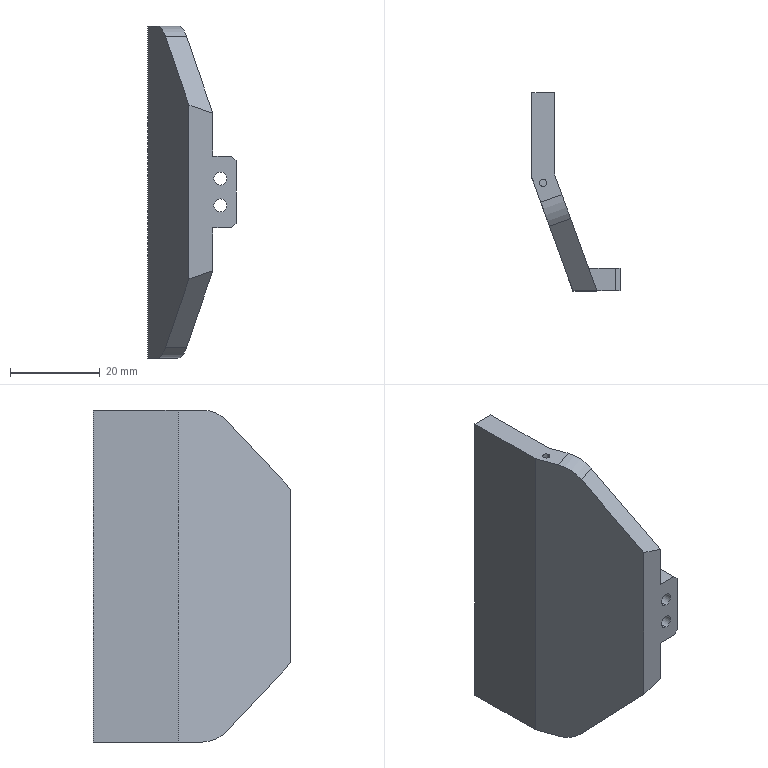NC program | NX | posted with a generic post | part box 19.643 x 44.061 x 74 mm
Whole program:
N10 G17 G21 G94 G90
(SPOT_FACING , TOOL : D4点钻)
N12 T05 M6
N14 G54
N16 G17 G0 G90 X0. Y-13. B0. C0. S3000 M3
N18 G43 Z30. H5
N20 G94 G82 G99 Z-1. F200. P200 R2.
N22 G80
N24 G0 X0. Y-13. Z30.
N26 M5
(SPOT_FACING_COPY , TOOL : D1.8钻头)
N28 T09 M6
N30 G54
N32 G17 G0 G90 X0. Y-13. B0. C0. S3000 M3
N34 G43 Z30. H9
N36 G94 G83 G99 Z-8. F150. Q1. R2.
N38 G80
N40 G0 X0. Y-13. Z30.
N42 M5
N44 M2